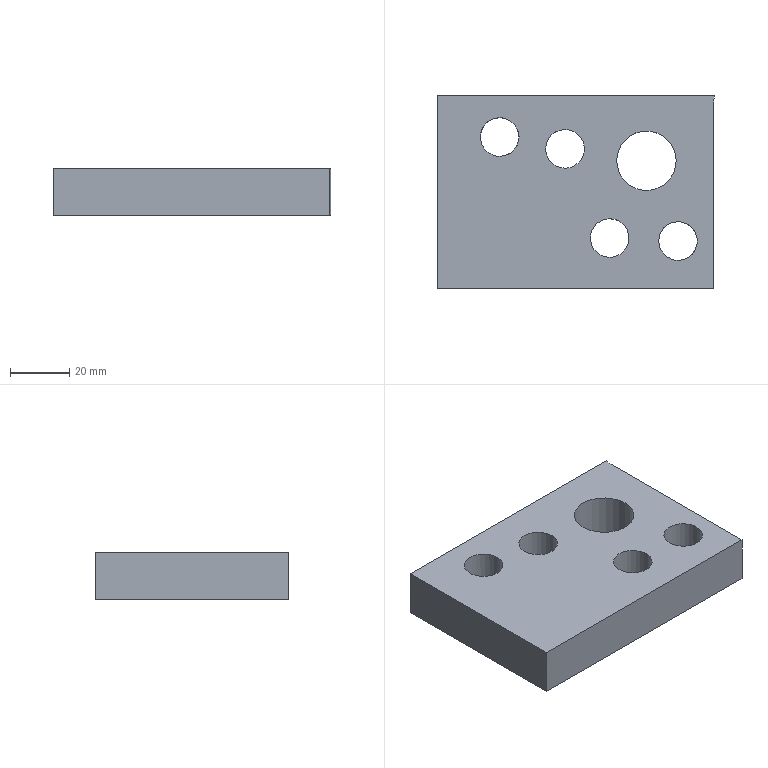Part | STEP file | gslz 2016.10.28-13_id746_x_t | 1 solid | 12 faces | box 93.344 x 65 x 16 mm | volume 83204 mm3 | plane 6 | cylinder 6 | commonest cylinder face diameters 13 x4 20 x1 22 x1
STEP:
#1=CARTESIAN_POINT('',(0.,0.,0.));
#2=DIRECTION('',(0.,0.,1.));
#3=DIRECTION('',(1.,0.,0.));
#4=AXIS2_PLACEMENT_3D('',#1,#2,#3);
#5=CARTESIAN_POINT('',(-1401.656,89.,-32.));
#6=VERTEX_POINT('',#5);
#7=CARTESIAN_POINT('',(-1495.,89.,-32.));
#8=VERTEX_POINT('',#7);
#9=CARTESIAN_POINT('',(-1374.,89.,-32.));
#10=DIRECTION('',(-1.,0.,0.));
#11=VECTOR('',#10,1.);
#12=LINE('',#9,#11);
#13=CARTESIAN_POINT('',(-1374.,128.728,-32.));
#14=DIRECTION('',(0.,0.,1.));
#15=DIRECTION('',(1.,0.,0.));
#16=AXIS2_PLACEMENT_3D('',#13,#14,#15);
#17=PLANE('',#16);
#18=CARTESIAN_POINT('',(0.,-39.728));
#19=DIRECTION('',(-1.,0.));
#20=VECTOR('',#19,1.);
#21=LINE('',#18,#20);
#22=(GEOMETRIC_REPRESENTATION_CONTEXT(2)PARAMETRIC_REPRESENTATION_CONTEXT()REPRESENTATION_CONTEXT('',''));
#23=DEFINITIONAL_REPRESENTATION('',(#21),#22);
#24=PCURVE('',#17,#23);
#25=CARTESIAN_POINT('',(-1448.,89.,-12.));
#26=DIRECTION('',(0.,-1.,0.));
#27=DIRECTION('',(0.,0.,-1.));
#28=AXIS2_PLACEMENT_3D('',#25,#26,#27);
#29=PLANE('',#28);
#30=CARTESIAN_POINT('',(20.,74.));
#31=DIRECTION('',(0.,-1.));
#32=VECTOR('',#31,1.);
#33=LINE('',#30,#32);
#34=(GEOMETRIC_REPRESENTATION_CONTEXT(2)PARAMETRIC_REPRESENTATION_CONTEXT()REPRESENTATION_CONTEXT('',''));
#35=DEFINITIONAL_REPRESENTATION('',(#33),#34);
#36=PCURVE('',#29,#35);
#37=SURFACE_CURVE('',#12,(#24,#36),.PCURVE_S1.);
#38=EDGE_CURVE('',#6,#8,#37,.T.);
#39=ORIENTED_EDGE('',*,*,#38,.T.);
#40=CARTESIAN_POINT('',(-1495.,24.,-32.));
#41=VERTEX_POINT('',#40);
#42=CARTESIAN_POINT('',(-1495.,220.,-32.));
#43=DIRECTION('',(0.,-1.,0.));
#44=VECTOR('',#43,1.);
#45=LINE('',#42,#44);
#46=CARTESIAN_POINT('',(-121.,91.272));
#47=DIRECTION('',(0.,-1.));
#48=VECTOR('',#47,1.);
#49=LINE('',#46,#48);
#50=(GEOMETRIC_REPRESENTATION_CONTEXT(2)PARAMETRIC_REPRESENTATION_CONTEXT()REPRESENTATION_CONTEXT('',''));
#51=DEFINITIONAL_REPRESENTATION('',(#49),#50);
#52=PCURVE('',#17,#51);
#53=CARTESIAN_POINT('',(-1495.,220.,-40.));
#54=DIRECTION('',(-1.,0.,0.));
#55=DIRECTION('',(0.,0.,1.));
#56=AXIS2_PLACEMENT_3D('',#53,#54,#55);
#57=PLANE('',#56);
#58=CARTESIAN_POINT('',(8.,0.));
#59=DIRECTION('',(0.,-1.));
#60=VECTOR('',#59,1.);
#61=LINE('',#58,#60);
#62=(GEOMETRIC_REPRESENTATION_CONTEXT(2)PARAMETRIC_REPRESENTATION_CONTEXT()REPRESENTATION_CONTEXT('',''));
#63=DEFINITIONAL_REPRESENTATION('',(#61),#62);
#64=PCURVE('',#57,#63);
#65=SURFACE_CURVE('',#45,(#52,#64),.PCURVE_S1.);
#66=EDGE_CURVE('',#8,#41,#65,.T.);
#67=ORIENTED_EDGE('',*,*,#66,.T.);
#68=CARTESIAN_POINT('',(-1402.,24.,-32.));
#69=VERTEX_POINT('',#68);
#70=CARTESIAN_POINT('',(-1490.,24.,-32.));
#71=DIRECTION('',(1.,0.,0.));
#72=VECTOR('',#71,1.);
#73=LINE('',#70,#72);
#74=CARTESIAN_POINT('',(-116.,-104.728));
#75=DIRECTION('',(1.,0.));
#76=VECTOR('',#75,1.);
#77=LINE('',#74,#76);
#78=(GEOMETRIC_REPRESENTATION_CONTEXT(2)PARAMETRIC_REPRESENTATION_CONTEXT()REPRESENTATION_CONTEXT('',''));
#79=DEFINITIONAL_REPRESENTATION('',(#77),#78);
#80=PCURVE('',#17,#79);
#81=CARTESIAN_POINT('',(-1490.,24.,-40.));
#82=DIRECTION('',(0.,-1.,0.));
#83=DIRECTION('',(1.,0.,0.));
#84=AXIS2_PLACEMENT_3D('',#81,#82,#83);
#85=PLANE('',#84);
#86=CARTESIAN_POINT('',(0.,8.));
#87=DIRECTION('',(1.,0.));
#88=VECTOR('',#87,1.);
#89=LINE('',#86,#88);
#90=(GEOMETRIC_REPRESENTATION_CONTEXT(2)PARAMETRIC_REPRESENTATION_CONTEXT()REPRESENTATION_CONTEXT('',''));
#91=DEFINITIONAL_REPRESENTATION('',(#89),#90);
#92=PCURVE('',#85,#91);
#93=SURFACE_CURVE('',#73,(#80,#92),.PCURVE_S1.);
#94=EDGE_CURVE('',#41,#69,#93,.T.);
#95=ORIENTED_EDGE('',*,*,#94,.T.);
#96=CARTESIAN_POINT('',(-1402.,86.272,-32.));
#97=VERTEX_POINT('',#96);
#98=CARTESIAN_POINT('',(-1402.,128.728,-32.));
#99=DIRECTION('',(0.,1.,0.));
#100=VECTOR('',#99,1.);
#101=LINE('',#98,#100);
#102=CARTESIAN_POINT('',(-28.,0.));
#103=DIRECTION('',(0.,1.));
#104=VECTOR('',#103,1.);
#105=LINE('',#102,#104);
#106=(GEOMETRIC_REPRESENTATION_CONTEXT(2)PARAMETRIC_REPRESENTATION_CONTEXT()REPRESENTATION_CONTEXT('',''));
#107=DEFINITIONAL_REPRESENTATION('',(#105),#106);
#108=PCURVE('',#17,#107);
#109=CARTESIAN_POINT('',(-1402.,30.,-40.));
#110=DIRECTION('',(1.,0.,0.));
#111=DIRECTION('',(0.,1.,0.));
#112=AXIS2_PLACEMENT_3D('',#109,#110,#111);
#113=PLANE('',#112);
#114=CARTESIAN_POINT('',(98.728,8.));
#115=DIRECTION('',(1.,0.));
#116=VECTOR('',#115,1.);
#117=LINE('',#114,#116);
#118=(GEOMETRIC_REPRESENTATION_CONTEXT(2)PARAMETRIC_REPRESENTATION_CONTEXT()REPRESENTATION_CONTEXT('',''));
#119=DEFINITIONAL_REPRESENTATION('',(#117),#118);
#120=PCURVE('',#113,#119);
#121=SURFACE_CURVE('',#101,(#108,#120),.PCURVE_S1.);
#122=EDGE_CURVE('',#69,#97,#121,.T.);
#123=ORIENTED_EDGE('',*,*,#122,.T.);
#124=CARTESIAN_POINT('',(-1391.,86.272,-32.));
#125=DIRECTION('',(0.,0.,-1.));
#126=DIRECTION('',(1.,0.,0.));
#127=AXIS2_PLACEMENT_3D('',#124,#125,#126);
#128=CIRCLE('',#127,11.);
#129=CARTESIAN_POINT('',(-6.,-42.456));
#130=CARTESIAN_POINT('',(-6.,-61.508));
#131=CARTESIAN_POINT('',(-22.5,-51.982));
#132=CARTESIAN_POINT('',(-39.,-42.456));
#133=CARTESIAN_POINT('',(-22.5,-32.93));
#134=CARTESIAN_POINT('',(-6.,-23.403));
#135=CARTESIAN_POINT('',(-6.,-42.456));
#136=(BOUNDED_CURVE()B_SPLINE_CURVE(2,(#129,#130,#131,#132,#133,#134,#135),.UNSPECIFIED.,.T.,.F.)B_SPLINE_CURVE_WITH_KNOTS((1,2,2,2,2,1),(-2.094,0.,2.094,4.189,6.283,8.378),.UNSPECIFIED.)CURVE()GEOMETRIC_REPRESENTATION_ITEM()RATIONAL_B_SPLINE_CURVE((1.,0.5,1.,0.5,1.,0.5,1.))REPRESENTATION_ITEM(''));
#137=(GEOMETRIC_REPRESENTATION_CONTEXT(2)PARAMETRIC_REPRESENTATION_CONTEXT()REPRESENTATION_CONTEXT('',''));
#138=DEFINITIONAL_REPRESENTATION('',(#136),#137);
#139=PCURVE('',#17,#138);
#140=CARTESIAN_POINT('',(-1391.,86.272,-40.));
#141=DIRECTION('',(0.,0.,1.));
#142=DIRECTION('',(1.,0.,0.));
#143=AXIS2_PLACEMENT_3D('',#140,#141,#142);
#144=CYLINDRICAL_SURFACE('',#143,11.);
#145=CARTESIAN_POINT('',(6.283,8.));
#146=DIRECTION('',(-1.,0.));
#147=VECTOR('',#146,1.);
#148=LINE('',#145,#147);
#149=(GEOMETRIC_REPRESENTATION_CONTEXT(2)PARAMETRIC_REPRESENTATION_CONTEXT()REPRESENTATION_CONTEXT('',''));
#150=DEFINITIONAL_REPRESENTATION('',(#148),#149);
#151=PCURVE('',#144,#150);
#152=SURFACE_CURVE('',#128,(#139,#151),.PCURVE_S1.);
#153=EDGE_CURVE('',#97,#6,#152,.T.);
#154=ORIENTED_EDGE('',*,*,#153,.T.);
#155=EDGE_LOOP('',(#39,#67,#95,#123,#154));
#156=FACE_BOUND('',#155,.T.);
#157=CARTESIAN_POINT('',(-1435.568,47.34,-32.));
#158=VERTEX_POINT('',#157);
#159=CARTESIAN_POINT('',(-1437.,41.,-32.));
#160=DIRECTION('',(0.,0.,-1.));
#161=DIRECTION('',(0.2202,0.9754,0.));
#162=AXIS2_PLACEMENT_3D('',#159,#160,#161);
#163=CIRCLE('',#162,6.5);
#164=CARTESIAN_POINT('',(-61.568,-81.388));
#165=CARTESIAN_POINT('',(-50.587,-83.867));
#166=CARTESIAN_POINT('',(-58.225,-92.138));
#167=CARTESIAN_POINT('',(-65.863,-100.409));
#168=CARTESIAN_POINT('',(-69.207,-89.658));
#169=CARTESIAN_POINT('',(-72.55,-78.908));
#170=CARTESIAN_POINT('',(-61.568,-81.388));
#171=(BOUNDED_CURVE()B_SPLINE_CURVE(2,(#164,#165,#166,#167,#168,#169,#170),.UNSPECIFIED.,.T.,.F.)B_SPLINE_CURVE_WITH_KNOTS((1,2,2,2,2,1),(-2.094,0.,2.094,4.189,6.283,8.378),.UNSPECIFIED.)CURVE()GEOMETRIC_REPRESENTATION_ITEM()RATIONAL_B_SPLINE_CURVE((1.,0.5,1.,0.5,1.,0.5,1.))REPRESENTATION_ITEM(''));
#172=(GEOMETRIC_REPRESENTATION_CONTEXT(2)PARAMETRIC_REPRESENTATION_CONTEXT()REPRESENTATION_CONTEXT('',''));
#173=DEFINITIONAL_REPRESENTATION('',(#171),#172);
#174=PCURVE('',#17,#173);
#175=CARTESIAN_POINT('',(-1437.,41.,-95.));
#176=DIRECTION('',(0.,0.,1.));
#177=DIRECTION('',(-0.2202,-0.9754,0.));
#178=AXIS2_PLACEMENT_3D('',#175,#176,#177);
#179=CYLINDRICAL_SURFACE('',#178,6.5);
#180=CARTESIAN_POINT('',(9.425,63.));
#181=DIRECTION('',(-1.,0.));
#182=VECTOR('',#181,1.);
#183=LINE('',#180,#182);
#184=(GEOMETRIC_REPRESENTATION_CONTEXT(2)PARAMETRIC_REPRESENTATION_CONTEXT()REPRESENTATION_CONTEXT('',''));
#185=DEFINITIONAL_REPRESENTATION('',(#183),#184);
#186=PCURVE('',#179,#185);
#187=SURFACE_CURVE('',#163,(#174,#186),.PCURVE_S1.);
#188=EDGE_CURVE('',#158,#158,#187,.T.);
#189=ORIENTED_EDGE('',*,*,#188,.T.);
#190=EDGE_LOOP('',(#189));
#191=FACE_BOUND('',#190,.T.);
#192=CARTESIAN_POINT('',(-1414.627,66.996,-32.));
#193=VERTEX_POINT('',#192);
#194=CARTESIAN_POINT('',(-1424.627,66.996,-32.));
#195=DIRECTION('',(0.,0.,1.));
#196=DIRECTION('',(1.,0.,0.));
#197=AXIS2_PLACEMENT_3D('',#194,#195,#196);
#198=CIRCLE('',#197,10.);
#199=CARTESIAN_POINT('',(-50.627,-61.732));
#200=DIRECTION('',(1.,0.));
#201=AXIS2_PLACEMENT_2D('',#199,#200);
#202=CIRCLE('',#201,10.);
#203=(GEOMETRIC_REPRESENTATION_CONTEXT(2)PARAMETRIC_REPRESENTATION_CONTEXT()REPRESENTATION_CONTEXT('',''));
#204=DEFINITIONAL_REPRESENTATION('',(#202),#203);
#205=PCURVE('',#17,#204);
#206=CARTESIAN_POINT('',(-1424.627,66.996,-82.));
#207=DIRECTION('',(0.,0.,1.));
#208=DIRECTION('',(1.,0.,0.));
#209=AXIS2_PLACEMENT_3D('',#206,#207,#208);
#210=CYLINDRICAL_SURFACE('',#209,10.);
#211=CARTESIAN_POINT('',(0.,50.));
#212=DIRECTION('',(1.,0.));
#213=VECTOR('',#212,1.);
#214=LINE('',#211,#213);
#215=(GEOMETRIC_REPRESENTATION_CONTEXT(2)PARAMETRIC_REPRESENTATION_CONTEXT()REPRESENTATION_CONTEXT('',''));
#216=DEFINITIONAL_REPRESENTATION('',(#214),#215);
#217=PCURVE('',#210,#216);
#218=SURFACE_CURVE('',#198,(#205,#217),.PCURVE_S1.);
#219=EDGE_CURVE('',#193,#193,#218,.T.);
#220=ORIENTED_EDGE('',*,*,#219,.F.);
#221=EDGE_LOOP('',(#220));
#222=FACE_BOUND('',#221,.T.);
#223=CARTESIAN_POINT('',(-1467.5,75.,-32.));
#224=VERTEX_POINT('',#223);
#225=CARTESIAN_POINT('',(-1475.091,68.592,-32.));
#226=VERTEX_POINT('',#225);
#227=CARTESIAN_POINT('',(-1474.,75.,-32.));
#228=DIRECTION('',(0.,0.,1.));
#229=DIRECTION('',(1.,0.,0.));
#230=AXIS2_PLACEMENT_3D('',#227,#228,#229);
#231=CIRCLE('',#230,6.5);
#232=CARTESIAN_POINT('',(-100.,-53.728));
#233=DIRECTION('',(1.,0.));
#234=AXIS2_PLACEMENT_2D('',#232,#233);
#235=CIRCLE('',#234,6.5);
#236=(GEOMETRIC_REPRESENTATION_CONTEXT(2)PARAMETRIC_REPRESENTATION_CONTEXT()REPRESENTATION_CONTEXT('',''));
#237=DEFINITIONAL_REPRESENTATION('',(#235),#236);
#238=PCURVE('',#17,#237);
#239=CARTESIAN_POINT('',(-1474.,75.,-0.5408));
#240=DIRECTION('',(0.,0.,-1.));
#241=DIRECTION('',(-1.,0.,0.));
#242=AXIS2_PLACEMENT_3D('',#239,#240,#241);
#243=CYLINDRICAL_SURFACE('',#242,6.5);
#244=CARTESIAN_POINT('',(9.425,31.459));
#245=DIRECTION('',(-1.,0.));
#246=VECTOR('',#245,1.);
#247=LINE('',#244,#246);
#248=(GEOMETRIC_REPRESENTATION_CONTEXT(2)PARAMETRIC_REPRESENTATION_CONTEXT()REPRESENTATION_CONTEXT('',''));
#249=DEFINITIONAL_REPRESENTATION('',(#247),#248);
#250=PCURVE('',#243,#249);
#251=SURFACE_CURVE('',#231,(#238,#250),.PCURVE_S1.);
#252=EDGE_CURVE('',#224,#226,#251,.T.);
#253=ORIENTED_EDGE('',*,*,#252,.F.);
#254=CARTESIAN_POINT('',(-1474.,75.,-32.));
#255=DIRECTION('',(0.,0.,1.));
#256=DIRECTION('',(1.,0.,0.));
#257=AXIS2_PLACEMENT_3D('',#254,#255,#256);
#258=CIRCLE('',#257,6.5);
#259=CARTESIAN_POINT('',(-100.,-53.728));
#260=DIRECTION('',(1.,0.));
#261=AXIS2_PLACEMENT_2D('',#259,#260);
#262=CIRCLE('',#261,6.5);
#263=(GEOMETRIC_REPRESENTATION_CONTEXT(2)PARAMETRIC_REPRESENTATION_CONTEXT()REPRESENTATION_CONTEXT('',''));
#264=DEFINITIONAL_REPRESENTATION('',(#262),#263);
#265=PCURVE('',#17,#264);
#266=CARTESIAN_POINT('',(15.708,31.459));
#267=DIRECTION('',(-1.,0.));
#268=VECTOR('',#267,1.);
#269=LINE('',#266,#268);
#270=(GEOMETRIC_REPRESENTATION_CONTEXT(2)PARAMETRIC_REPRESENTATION_CONTEXT()REPRESENTATION_CONTEXT('',''));
#271=DEFINITIONAL_REPRESENTATION('',(#269),#270);
#272=PCURVE('',#243,#271);
#273=SURFACE_CURVE('',#258,(#265,#272),.PCURVE_S1.);
#274=EDGE_CURVE('',#226,#224,#273,.T.);
#275=ORIENTED_EDGE('',*,*,#274,.F.);
#276=EDGE_LOOP('',(#253,#275));
#277=FACE_BOUND('',#276,.T.);
#278=CARTESIAN_POINT('',(-1450.568,77.34,-32.));
#279=VERTEX_POINT('',#278);
#280=CARTESIAN_POINT('',(-1452.,71.,-32.));
#281=DIRECTION('',(0.,0.,-1.));
#282=DIRECTION('',(0.2202,0.9754,0.));
#283=AXIS2_PLACEMENT_3D('',#280,#281,#282);
#284=CIRCLE('',#283,6.5);
#285=CARTESIAN_POINT('',(-76.568,-51.388));
#286=CARTESIAN_POINT('',(-65.587,-53.867));
#287=CARTESIAN_POINT('',(-73.225,-62.138));
#288=CARTESIAN_POINT('',(-80.863,-70.409));
#289=CARTESIAN_POINT('',(-84.207,-59.658));
#290=CARTESIAN_POINT('',(-87.55,-48.908));
#291=CARTESIAN_POINT('',(-76.568,-51.388));
#292=(BOUNDED_CURVE()B_SPLINE_CURVE(2,(#285,#286,#287,#288,#289,#290,#291),.UNSPECIFIED.,.T.,.F.)B_SPLINE_CURVE_WITH_KNOTS((1,2,2,2,2,1),(-2.094,0.,2.094,4.189,6.283,8.378),.UNSPECIFIED.)CURVE()GEOMETRIC_REPRESENTATION_ITEM()RATIONAL_B_SPLINE_CURVE((1.,0.5,1.,0.5,1.,0.5,1.))REPRESENTATION_ITEM(''));
#293=(GEOMETRIC_REPRESENTATION_CONTEXT(2)PARAMETRIC_REPRESENTATION_CONTEXT()REPRESENTATION_CONTEXT('',''));
#294=DEFINITIONAL_REPRESENTATION('',(#292),#293);
#295=PCURVE('',#17,#294);
#296=CARTESIAN_POINT('',(-1452.,71.,-95.));
#297=DIRECTION('',(0.,0.,1.));
#298=DIRECTION('',(-0.2202,-0.9754,0.));
#299=AXIS2_PLACEMENT_3D('',#296,#297,#298);
#300=CYLINDRICAL_SURFACE('',#299,6.5);
#301=CARTESIAN_POINT('',(9.425,63.));
#302=DIRECTION('',(-1.,0.));
#303=VECTOR('',#302,1.);
#304=LINE('',#301,#303);
#305=(GEOMETRIC_REPRESENTATION_CONTEXT(2)PARAMETRIC_REPRESENTATION_CONTEXT()REPRESENTATION_CONTEXT('',''));
#306=DEFINITIONAL_REPRESENTATION('',(#304),#305);
#307=PCURVE('',#300,#306);
#308=SURFACE_CURVE('',#284,(#295,#307),.PCURVE_S1.);
#309=EDGE_CURVE('',#279,#279,#308,.T.);
#310=ORIENTED_EDGE('',*,*,#309,.T.);
#311=EDGE_LOOP('',(#310));
#312=FACE_BOUND('',#311,.T.);
#313=CARTESIAN_POINT('',(-1407.5,40.,-32.));
#314=VERTEX_POINT('',#313);
#315=CARTESIAN_POINT('',(-1415.091,33.592,-32.));
#316=VERTEX_POINT('',#315);
#317=CARTESIAN_POINT('',(-1414.,40.,-32.));
#318=DIRECTION('',(0.,0.,1.));
#319=DIRECTION('',(1.,0.,0.));
#320=AXIS2_PLACEMENT_3D('',#317,#318,#319);
#321=CIRCLE('',#320,6.5);
#322=CARTESIAN_POINT('',(-40.,-88.728));
#323=DIRECTION('',(1.,0.));
#324=AXIS2_PLACEMENT_2D('',#322,#323);
#325=CIRCLE('',#324,6.5);
#326=(GEOMETRIC_REPRESENTATION_CONTEXT(2)PARAMETRIC_REPRESENTATION_CONTEXT()REPRESENTATION_CONTEXT('',''));
#327=DEFINITIONAL_REPRESENTATION('',(#325),#326);
#328=PCURVE('',#17,#327);
#329=CARTESIAN_POINT('',(-1414.,40.,-0.5408));
#330=DIRECTION('',(0.,0.,-1.));
#331=DIRECTION('',(-1.,0.,0.));
#332=AXIS2_PLACEMENT_3D('',#329,#330,#331);
#333=CYLINDRICAL_SURFACE('',#332,6.5);
#334=CARTESIAN_POINT('',(9.425,31.459));
#335=DIRECTION('',(-1.,0.));
#336=VECTOR('',#335,1.);
#337=LINE('',#334,#336);
#338=(GEOMETRIC_REPRESENTATION_CONTEXT(2)PARAMETRIC_REPRESENTATION_CONTEXT()REPRESENTATION_CONTEXT('',''));
#339=DEFINITIONAL_REPRESENTATION('',(#337),#338);
#340=PCURVE('',#333,#339);
#341=SURFACE_CURVE('',#321,(#328,#340),.PCURVE_S1.);
#342=EDGE_CURVE('',#314,#316,#341,.T.);
#343=ORIENTED_EDGE('',*,*,#342,.F.);
#344=CARTESIAN_POINT('',(-1414.,40.,-32.));
#345=DIRECTION('',(0.,0.,1.));
#346=DIRECTION('',(1.,0.,0.));
#347=AXIS2_PLACEMENT_3D('',#344,#345,#346);
#348=CIRCLE('',#347,6.5);
#349=CARTESIAN_POINT('',(-40.,-88.728));
#350=DIRECTION('',(1.,0.));
#351=AXIS2_PLACEMENT_2D('',#349,#350);
#352=CIRCLE('',#351,6.5);
#353=(GEOMETRIC_REPRESENTATION_CONTEXT(2)PARAMETRIC_REPRESENTATION_CONTEXT()REPRESENTATION_CONTEXT('',''));
#354=DEFINITIONAL_REPRESENTATION('',(#352),#353);
#355=PCURVE('',#17,#354);
#356=CARTESIAN_POINT('',(15.708,31.459));
#357=DIRECTION('',(-1.,0.));
#358=VECTOR('',#357,1.);
#359=LINE('',#356,#358);
#360=(GEOMETRIC_REPRESENTATION_CONTEXT(2)PARAMETRIC_REPRESENTATION_CONTEXT()REPRESENTATION_CONTEXT('',''));
#361=DEFINITIONAL_REPRESENTATION('',(#359),#360);
#362=PCURVE('',#333,#361);
#363=SURFACE_CURVE('',#348,(#355,#362),.PCURVE_S1.);
#364=EDGE_CURVE('',#316,#314,#363,.T.);
#365=ORIENTED_EDGE('',*,*,#364,.F.);
#366=EDGE_LOOP('',(#343,#365));
#367=FACE_BOUND('',#366,.T.);
#368=ADVANCED_FACE('',(#156,#191,#222,#277,#312,#367),#17,.T.);
#369=CARTESIAN_POINT('',(-1415.091,33.592,-48.));
#370=VERTEX_POINT('',#369);
#371=CARTESIAN_POINT('',(-1414.,40.,-48.));
#372=DIRECTION('',(0.,0.,1.));
#373=DIRECTION('',(-0.1678,-0.9858,0.));
#374=AXIS2_PLACEMENT_3D('',#371,#372,#373);
#375=CIRCLE('',#374,6.5);
#376=CARTESIAN_POINT('',(-1374.,128.728,-48.));
#377=DIRECTION('',(0.,0.,1.));
#378=DIRECTION('',(1.,0.,0.));
#379=AXIS2_PLACEMENT_3D('',#376,#377,#378);
#380=PLANE('',#379);
#381=CARTESIAN_POINT('',(-40.,-88.728));
#382=DIRECTION('',(-0.1678,-0.9858));
#383=AXIS2_PLACEMENT_2D('',#381,#382);
#384=CIRCLE('',#383,6.5);
#385=(GEOMETRIC_REPRESENTATION_CONTEXT(2)PARAMETRIC_REPRESENTATION_CONTEXT()REPRESENTATION_CONTEXT('',''));
#386=DEFINITIONAL_REPRESENTATION('',(#384),#385);
#387=PCURVE('',#380,#386);
#388=CARTESIAN_POINT('',(11.164,47.459));
#389=DIRECTION('',(-1.,0.));
#390=VECTOR('',#389,1.);
#391=LINE('',#388,#390);
#392=(GEOMETRIC_REPRESENTATION_CONTEXT(2)PARAMETRIC_REPRESENTATION_CONTEXT()REPRESENTATION_CONTEXT('',''));
#393=DEFINITIONAL_REPRESENTATION('',(#391),#392);
#394=PCURVE('',#333,#393);
#395=SURFACE_CURVE('',#375,(#387,#394),.PCURVE_S1.);
#396=EDGE_CURVE('',#370,#370,#395,.T.);
#397=ORIENTED_EDGE('',*,*,#396,.T.);
#398=EDGE_LOOP('',(#397));
#399=FACE_BOUND('',#398,.T.);
#400=CARTESIAN_POINT('',(-1435.568,47.34,-48.));
#401=VERTEX_POINT('',#400);
#402=CARTESIAN_POINT('',(-1437.,41.,-48.));
#403=DIRECTION('',(0.,0.,1.));
#404=DIRECTION('',(0.2202,0.9754,0.));
#405=AXIS2_PLACEMENT_3D('',#402,#403,#404);
#406=CIRCLE('',#405,6.5);
#407=CARTESIAN_POINT('',(-63.,-87.728));
#408=DIRECTION('',(0.2202,0.9754));
#409=AXIS2_PLACEMENT_2D('',#407,#408);
#410=CIRCLE('',#409,6.5);
#411=(GEOMETRIC_REPRESENTATION_CONTEXT(2)PARAMETRIC_REPRESENTATION_CONTEXT()REPRESENTATION_CONTEXT('',''));
#412=DEFINITIONAL_REPRESENTATION('',(#410),#411);
#413=PCURVE('',#380,#412);
#414=CARTESIAN_POINT('',(3.142,47.));
#415=DIRECTION('',(1.,0.));
#416=VECTOR('',#415,1.);
#417=LINE('',#414,#416);
#418=(GEOMETRIC_REPRESENTATION_CONTEXT(2)PARAMETRIC_REPRESENTATION_CONTEXT()REPRESENTATION_CONTEXT('',''));
#419=DEFINITIONAL_REPRESENTATION('',(#417),#418);
#420=PCURVE('',#179,#419);
#421=SURFACE_CURVE('',#406,(#413,#420),.PCURVE_S1.);
#422=EDGE_CURVE('',#401,#401,#421,.T.);
#423=ORIENTED_EDGE('',*,*,#422,.T.);
#424=EDGE_LOOP('',(#423));
#425=FACE_BOUND('',#424,.T.);
#426=CARTESIAN_POINT('',(-1450.568,77.34,-48.));
#427=VERTEX_POINT('',#426);
#428=CARTESIAN_POINT('',(-1452.,71.,-48.));
#429=DIRECTION('',(0.,0.,1.));
#430=DIRECTION('',(0.2202,0.9754,0.));
#431=AXIS2_PLACEMENT_3D('',#428,#429,#430);
#432=CIRCLE('',#431,6.5);
#433=CARTESIAN_POINT('',(-78.,-57.728));
#434=DIRECTION('',(0.2202,0.9754));
#435=AXIS2_PLACEMENT_2D('',#433,#434);
#436=CIRCLE('',#435,6.5);
#437=(GEOMETRIC_REPRESENTATION_CONTEXT(2)PARAMETRIC_REPRESENTATION_CONTEXT()REPRESENTATION_CONTEXT('',''));
#438=DEFINITIONAL_REPRESENTATION('',(#436),#437);
#439=PCURVE('',#380,#438);
#440=CARTESIAN_POINT('',(3.142,47.));
#441=DIRECTION('',(1.,0.));
#442=VECTOR('',#441,1.);
#443=LINE('',#440,#442);
#444=(GEOMETRIC_REPRESENTATION_CONTEXT(2)PARAMETRIC_REPRESENTATION_CONTEXT()REPRESENTATION_CONTEXT('',''));
#445=DEFINITIONAL_REPRESENTATION('',(#443),#444);
#446=PCURVE('',#300,#445);
#447=SURFACE_CURVE('',#432,(#439,#446),.PCURVE_S1.);
#448=EDGE_CURVE('',#427,#427,#447,.T.);
#449=ORIENTED_EDGE('',*,*,#448,.T.);
#450=EDGE_LOOP('',(#449));
#451=FACE_BOUND('',#450,.T.);
#452=CARTESIAN_POINT('',(-1475.091,68.592,-48.));
#453=VERTEX_POINT('',#452);
#454=CARTESIAN_POINT('',(-1474.,75.,-48.));
#455=DIRECTION('',(0.,0.,1.));
#456=DIRECTION('',(-0.1678,-0.9858,0.));
#457=AXIS2_PLACEMENT_3D('',#454,#455,#456);
#458=CIRCLE('',#457,6.5);
#459=CARTESIAN_POINT('',(-100.,-53.728));
#460=DIRECTION('',(-0.1678,-0.9858));
#461=AXIS2_PLACEMENT_2D('',#459,#460);
#462=CIRCLE('',#461,6.5);
#463=(GEOMETRIC_REPRESENTATION_CONTEXT(2)PARAMETRIC_REPRESENTATION_CONTEXT()REPRESENTATION_CONTEXT('',''));
#464=DEFINITIONAL_REPRESENTATION('',(#462),#463);
#465=PCURVE('',#380,#464);
#466=CARTESIAN_POINT('',(11.164,47.459));
#467=DIRECTION('',(-1.,0.));
#468=VECTOR('',#467,1.);
#469=LINE('',#466,#468);
#470=(GEOMETRIC_REPRESENTATION_CONTEXT(2)PARAMETRIC_REPRESENTATION_CONTEXT()REPRESENTATION_CONTEXT('',''));
#471=DEFINITIONAL_REPRESENTATION('',(#469),#470);
#472=PCURVE('',#243,#471);
#473=SURFACE_CURVE('',#458,(#465,#472),.PCURVE_S1.);
#474=EDGE_CURVE('',#453,#453,#473,.T.);
#475=ORIENTED_EDGE('',*,*,#474,.T.);
#476=EDGE_LOOP('',(#475));
#477=FACE_BOUND('',#476,.T.);
#478=CARTESIAN_POINT('',(-1414.627,66.996,-48.));
#479=VERTEX_POINT('',#478);
#480=CARTESIAN_POINT('',(-1424.627,66.996,-48.));
#481=DIRECTION('',(0.,0.,1.));
#482=DIRECTION('',(1.,0.,0.));
#483=AXIS2_PLACEMENT_3D('',#480,#481,#482);
#484=CIRCLE('',#483,10.);
#485=CARTESIAN_POINT('',(-50.627,-61.732));
#486=DIRECTION('',(1.,0.));
#487=AXIS2_PLACEMENT_2D('',#485,#486);
#488=CIRCLE('',#487,10.);
#489=(GEOMETRIC_REPRESENTATION_CONTEXT(2)PARAMETRIC_REPRESENTATION_CONTEXT()REPRESENTATION_CONTEXT('',''));
#490=DEFINITIONAL_REPRESENTATION('',(#488),#489);
#491=PCURVE('',#380,#490);
#492=CARTESIAN_POINT('',(0.,34.));
#493=DIRECTION('',(1.,0.));
#494=VECTOR('',#493,1.);
#495=LINE('',#492,#494);
#496=(GEOMETRIC_REPRESENTATION_CONTEXT(2)PARAMETRIC_REPRESENTATION_CONTEXT()REPRESENTATION_CONTEXT('',''));
#497=DEFINITIONAL_REPRESENTATION('',(#495),#496);
#498=PCURVE('',#210,#497);
#499=SURFACE_CURVE('',#484,(#491,#498),.PCURVE_S1.);
#500=EDGE_CURVE('',#479,#479,#499,.T.);
#501=ORIENTED_EDGE('',*,*,#500,.T.);
#502=EDGE_LOOP('',(#501));
#503=FACE_BOUND('',#502,.T.);
#504=CARTESIAN_POINT('',(-1495.,89.,-48.));
#505=VERTEX_POINT('',#504);
#506=CARTESIAN_POINT('',(-1495.,24.,-48.));
#507=VERTEX_POINT('',#506);
#508=CARTESIAN_POINT('',(-1495.,220.,-48.));
#509=DIRECTION('',(0.,-1.,0.));
#510=VECTOR('',#509,1.);
#511=LINE('',#508,#510);
#512=CARTESIAN_POINT('',(-121.,91.272));
#513=DIRECTION('',(0.,-1.));
#514=VECTOR('',#513,1.);
#515=LINE('',#512,#514);
#516=(GEOMETRIC_REPRESENTATION_CONTEXT(2)PARAMETRIC_REPRESENTATION_CONTEXT()REPRESENTATION_CONTEXT('',''));
#517=DEFINITIONAL_REPRESENTATION('',(#515),#516);
#518=PCURVE('',#380,#517);
#519=CARTESIAN_POINT('',(-8.,0.));
#520=DIRECTION('',(0.,-1.));
#521=VECTOR('',#520,1.);
#522=LINE('',#519,#521);
#523=(GEOMETRIC_REPRESENTATION_CONTEXT(2)PARAMETRIC_REPRESENTATION_CONTEXT()REPRESENTATION_CONTEXT('',''));
#524=DEFINITIONAL_REPRESENTATION('',(#522),#523);
#525=PCURVE('',#57,#524);
#526=SURFACE_CURVE('',#511,(#518,#525),.PCURVE_S1.);
#527=EDGE_CURVE('',#505,#507,#526,.T.);
#528=ORIENTED_EDGE('',*,*,#527,.F.);
#529=CARTESIAN_POINT('',(-1401.656,89.,-48.));
#530=VERTEX_POINT('',#529);
#531=CARTESIAN_POINT('',(-1374.,89.,-48.));
#532=DIRECTION('',(-1.,0.,0.));
#533=VECTOR('',#532,1.);
#534=LINE('',#531,#533);
#535=CARTESIAN_POINT('',(0.,-39.728));
#536=DIRECTION('',(-1.,0.));
#537=VECTOR('',#536,1.);
#538=LINE('',#535,#537);
#539=(GEOMETRIC_REPRESENTATION_CONTEXT(2)PARAMETRIC_REPRESENTATION_CONTEXT()REPRESENTATION_CONTEXT('',''));
#540=DEFINITIONAL_REPRESENTATION('',(#538),#539);
#541=PCURVE('',#380,#540);
#542=CARTESIAN_POINT('',(36.,74.));
#543=DIRECTION('',(0.,-1.));
#544=VECTOR('',#543,1.);
#545=LINE('',#542,#544);
#546=(GEOMETRIC_REPRESENTATION_CONTEXT(2)PARAMETRIC_REPRESENTATION_CONTEXT()REPRESENTATION_CONTEXT('',''));
#547=DEFINITIONAL_REPRESENTATION('',(#545),#546);
#548=PCURVE('',#29,#547);
#549=SURFACE_CURVE('',#534,(#541,#548),.PCURVE_S1.);
#550=EDGE_CURVE('',#530,#505,#549,.T.);
#551=ORIENTED_EDGE('',*,*,#550,.F.);
#552=CARTESIAN_POINT('',(-1402.,86.272,-48.));
#553=VERTEX_POINT('',#552);
#554=CARTESIAN_POINT('',(-1391.,86.272,-48.));
#555=DIRECTION('',(0.,0.,-1.));
#556=DIRECTION('',(1.,0.,0.));
#557=AXIS2_PLACEMENT_3D('',#554,#555,#556);
#558=CIRCLE('',#557,11.);
#559=CARTESIAN_POINT('',(-6.,-42.456));
#560=CARTESIAN_POINT('',(-6.,-61.508));
#561=CARTESIAN_POINT('',(-22.5,-51.982));
#562=CARTESIAN_POINT('',(-39.,-42.456));
#563=CARTESIAN_POINT('',(-22.5,-32.93));
#564=CARTESIAN_POINT('',(-6.,-23.403));
#565=CARTESIAN_POINT('',(-6.,-42.456));
#566=(BOUNDED_CURVE()B_SPLINE_CURVE(2,(#559,#560,#561,#562,#563,#564,#565),.UNSPECIFIED.,.T.,.F.)B_SPLINE_CURVE_WITH_KNOTS((1,2,2,2,2,1),(-2.094,0.,2.094,4.189,6.283,8.378),.UNSPECIFIED.)CURVE()GEOMETRIC_REPRESENTATION_ITEM()RATIONAL_B_SPLINE_CURVE((1.,0.5,1.,0.5,1.,0.5,1.))REPRESENTATION_ITEM(''));
#567=(GEOMETRIC_REPRESENTATION_CONTEXT(2)PARAMETRIC_REPRESENTATION_CONTEXT()REPRESENTATION_CONTEXT('',''));
#568=DEFINITIONAL_REPRESENTATION('',(#566),#567);
#569=PCURVE('',#380,#568);
#570=CARTESIAN_POINT('',(6.283,-8.));
#571=DIRECTION('',(-1.,0.));
#572=VECTOR('',#571,1.);
#573=LINE('',#570,#572);
#574=(GEOMETRIC_REPRESENTATION_CONTEXT(2)PARAMETRIC_REPRESENTATION_CONTEXT()REPRESENTATION_CONTEXT('',''));
#575=DEFINITIONAL_REPRESENTATION('',(#573),#574);
#576=PCURVE('',#144,#575);
#577=SURFACE_CURVE('',#558,(#569,#576),.PCURVE_S1.);
#578=EDGE_CURVE('',#553,#530,#577,.T.);
#579=ORIENTED_EDGE('',*,*,#578,.F.);
#580=CARTESIAN_POINT('',(-1402.,24.,-48.));
#581=VERTEX_POINT('',#580);
#582=CARTESIAN_POINT('',(-1402.,128.728,-48.));
#583=DIRECTION('',(0.,1.,0.));
#584=VECTOR('',#583,1.);
#585=LINE('',#582,#584);
#586=CARTESIAN_POINT('',(-28.,0.));
#587=DIRECTION('',(0.,1.));
#588=VECTOR('',#587,1.);
#589=LINE('',#586,#588);
#590=(GEOMETRIC_REPRESENTATION_CONTEXT(2)PARAMETRIC_REPRESENTATION_CONTEXT()REPRESENTATION_CONTEXT('',''));
#591=DEFINITIONAL_REPRESENTATION('',(#589),#590);
#592=PCURVE('',#380,#591);
#593=CARTESIAN_POINT('',(98.728,-8.));
#594=DIRECTION('',(1.,0.));
#595=VECTOR('',#594,1.);
#596=LINE('',#593,#595);
#597=(GEOMETRIC_REPRESENTATION_CONTEXT(2)PARAMETRIC_REPRESENTATION_CONTEXT()REPRESENTATION_CONTEXT('',''));
#598=DEFINITIONAL_REPRESENTATION('',(#596),#597);
#599=PCURVE('',#113,#598);
#600=SURFACE_CURVE('',#585,(#592,#599),.PCURVE_S1.);
#601=EDGE_CURVE('',#581,#553,#600,.T.);
#602=ORIENTED_EDGE('',*,*,#601,.F.);
#603=CARTESIAN_POINT('',(-1490.,24.,-48.));
#604=DIRECTION('',(1.,0.,0.));
#605=VECTOR('',#604,1.);
#606=LINE('',#603,#605);
#607=CARTESIAN_POINT('',(-116.,-104.728));
#608=DIRECTION('',(1.,0.));
#609=VECTOR('',#608,1.);
#610=LINE('',#607,#609);
#611=(GEOMETRIC_REPRESENTATION_CONTEXT(2)PARAMETRIC_REPRESENTATION_CONTEXT()REPRESENTATION_CONTEXT('',''));
#612=DEFINITIONAL_REPRESENTATION('',(#610),#611);
#613=PCURVE('',#380,#612);
#614=CARTESIAN_POINT('',(0.,-8.));
#615=DIRECTION('',(1.,0.));
#616=VECTOR('',#615,1.);
#617=LINE('',#614,#616);
#618=(GEOMETRIC_REPRESENTATION_CONTEXT(2)PARAMETRIC_REPRESENTATION_CONTEXT()REPRESENTATION_CONTEXT('',''));
#619=DEFINITIONAL_REPRESENTATION('',(#617),#618);
#620=PCURVE('',#85,#619);
#621=SURFACE_CURVE('',#606,(#613,#620),.PCURVE_S1.);
#622=EDGE_CURVE('',#507,#581,#621,.T.);
#623=ORIENTED_EDGE('',*,*,#622,.F.);
#624=EDGE_LOOP('',(#528,#551,#579,#602,#623));
#625=FACE_BOUND('',#624,.T.);
#626=ADVANCED_FACE('',(#399,#425,#451,#477,#503,#625),#380,.F.);
#627=ORIENTED_EDGE('',*,*,#578,.F.);
#628=CARTESIAN_POINT('',(-1402.,86.272,-40.));
#629=DIRECTION('',(0.,0.,1.));
#630=VECTOR('',#629,1.);
#631=LINE('',#628,#630);
#632=CARTESIAN_POINT('',(3.142,0.));
#633=DIRECTION('',(0.,1.));
#634=VECTOR('',#633,1.);
#635=LINE('',#632,#634);
#636=(GEOMETRIC_REPRESENTATION_CONTEXT(2)PARAMETRIC_REPRESENTATION_CONTEXT()REPRESENTATION_CONTEXT('',''));
#637=DEFINITIONAL_REPRESENTATION('',(#635),#636);
#638=PCURVE('',#144,#637);
#639=CARTESIAN_POINT('',(56.272,0.));
#640=DIRECTION('',(0.,1.));
#641=VECTOR('',#640,1.);
#642=LINE('',#639,#641);
#643=(GEOMETRIC_REPRESENTATION_CONTEXT(2)PARAMETRIC_REPRESENTATION_CONTEXT()REPRESENTATION_CONTEXT('',''));
#644=DEFINITIONAL_REPRESENTATION('',(#642),#643);
#645=PCURVE('',#113,#644);
#646=SURFACE_CURVE('',#631,(#638,#645),.PCURVE_S1.);
#647=EDGE_CURVE('',#553,#97,#646,.T.);
#648=ORIENTED_EDGE('',*,*,#647,.T.);
#649=ORIENTED_EDGE('',*,*,#153,.T.);
#650=CARTESIAN_POINT('',(-1401.656,89.,-40.));
#651=DIRECTION('',(0.,0.,1.));
#652=VECTOR('',#651,1.);
#653=LINE('',#650,#652);
#654=CARTESIAN_POINT('',(2.891,0.));
#655=DIRECTION('',(0.,1.));
#656=VECTOR('',#655,1.);
#657=LINE('',#654,#656);
#658=(GEOMETRIC_REPRESENTATION_CONTEXT(2)PARAMETRIC_REPRESENTATION_CONTEXT()REPRESENTATION_CONTEXT('',''));
#659=DEFINITIONAL_REPRESENTATION('',(#657),#658);
#660=PCURVE('',#144,#659);
#661=CARTESIAN_POINT('',(28.,46.344));
#662=DIRECTION('',(-1.,0.));
#663=VECTOR('',#662,1.);
#664=LINE('',#661,#663);
#665=(GEOMETRIC_REPRESENTATION_CONTEXT(2)PARAMETRIC_REPRESENTATION_CONTEXT()REPRESENTATION_CONTEXT('',''));
#666=DEFINITIONAL_REPRESENTATION('',(#664),#665);
#667=PCURVE('',#29,#666);
#668=SURFACE_CURVE('',#653,(#660,#667),.PCURVE_S1.);
#669=EDGE_CURVE('',#530,#6,#668,.T.);
#670=ORIENTED_EDGE('',*,*,#669,.F.);
#671=EDGE_LOOP('',(#627,#648,#649,#670));
#672=FACE_BOUND('',#671,.F.);
#673=ADVANCED_FACE('',(#672),#144,.F.);
#674=ORIENTED_EDGE('',*,*,#122,.F.);
#675=CARTESIAN_POINT('',(-1402.,24.,-40.));
#676=DIRECTION('',(0.,0.,1.));
#677=VECTOR('',#676,1.);
#678=LINE('',#675,#677);
#679=CARTESIAN_POINT('',(-6.,0.));
#680=DIRECTION('',(0.,1.));
#681=VECTOR('',#680,1.);
#682=LINE('',#679,#681);
#683=(GEOMETRIC_REPRESENTATION_CONTEXT(2)PARAMETRIC_REPRESENTATION_CONTEXT()REPRESENTATION_CONTEXT('',''));
#684=DEFINITIONAL_REPRESENTATION('',(#682),#683);
#685=PCURVE('',#113,#684);
#686=CARTESIAN_POINT('',(88.,0.));
#687=DIRECTION('',(0.,1.));
#688=VECTOR('',#687,1.);
#689=LINE('',#686,#688);
#690=(GEOMETRIC_REPRESENTATION_CONTEXT(2)PARAMETRIC_REPRESENTATION_CONTEXT()REPRESENTATION_CONTEXT('',''));
#691=DEFINITIONAL_REPRESENTATION('',(#689),#690);
#692=PCURVE('',#85,#691);
#693=SURFACE_CURVE('',#678,(#685,#692),.PCURVE_S1.);
#694=EDGE_CURVE('',#581,#69,#693,.T.);
#695=ORIENTED_EDGE('',*,*,#694,.F.);
#696=ORIENTED_EDGE('',*,*,#601,.T.);
#697=ORIENTED_EDGE('',*,*,#647,.T.);
#698=EDGE_LOOP('',(#674,#695,#696,#697));
#699=FACE_BOUND('',#698,.T.);
#700=ADVANCED_FACE('',(#699),#113,.T.);
#701=ORIENTED_EDGE('',*,*,#94,.F.);
#702=CARTESIAN_POINT('',(-1495.,24.,-40.));
#703=DIRECTION('',(0.,0.,1.));
#704=VECTOR('',#703,1.);
#705=LINE('',#702,#704);
#706=CARTESIAN_POINT('',(-5.,0.));
#707=DIRECTION('',(0.,1.));
#708=VECTOR('',#707,1.);
#709=LINE('',#706,#708);
#710=(GEOMETRIC_REPRESENTATION_CONTEXT(2)PARAMETRIC_REPRESENTATION_CONTEXT()REPRESENTATION_CONTEXT('',''));
#711=DEFINITIONAL_REPRESENTATION('',(#709),#710);
#712=PCURVE('',#85,#711);
#713=CARTESIAN_POINT('',(0.,-196.));
#714=DIRECTION('',(1.,0.));
#715=VECTOR('',#714,1.);
#716=LINE('',#713,#715);
#717=(GEOMETRIC_REPRESENTATION_CONTEXT(2)PARAMETRIC_REPRESENTATION_CONTEXT()REPRESENTATION_CONTEXT('',''));
#718=DEFINITIONAL_REPRESENTATION('',(#716),#717);
#719=PCURVE('',#57,#718);
#720=SURFACE_CURVE('',#705,(#712,#719),.PCURVE_S1.);
#721=EDGE_CURVE('',#507,#41,#720,.T.);
#722=ORIENTED_EDGE('',*,*,#721,.F.);
#723=ORIENTED_EDGE('',*,*,#622,.T.);
#724=ORIENTED_EDGE('',*,*,#694,.T.);
#725=EDGE_LOOP('',(#701,#722,#723,#724));
#726=FACE_BOUND('',#725,.T.);
#727=ADVANCED_FACE('',(#726),#85,.T.);
#728=CARTESIAN_POINT('',(-1495.,89.,-40.));
#729=DIRECTION('',(0.,0.,1.));
#730=VECTOR('',#729,1.);
#731=LINE('',#728,#730);
#732=CARTESIAN_POINT('',(0.,-131.));
#733=DIRECTION('',(1.,0.));
#734=VECTOR('',#733,1.);
#735=LINE('',#732,#734);
#736=(GEOMETRIC_REPRESENTATION_CONTEXT(2)PARAMETRIC_REPRESENTATION_CONTEXT()REPRESENTATION_CONTEXT('',''));
#737=DEFINITIONAL_REPRESENTATION('',(#735),#736);
#738=PCURVE('',#57,#737);
#739=CARTESIAN_POINT('',(28.,-47.));
#740=DIRECTION('',(-1.,0.));
#741=VECTOR('',#740,1.);
#742=LINE('',#739,#741);
#743=(GEOMETRIC_REPRESENTATION_CONTEXT(2)PARAMETRIC_REPRESENTATION_CONTEXT()REPRESENTATION_CONTEXT('',''));
#744=DEFINITIONAL_REPRESENTATION('',(#742),#743);
#745=PCURVE('',#29,#744);
#746=SURFACE_CURVE('',#731,(#738,#745),.PCURVE_S1.);
#747=EDGE_CURVE('',#505,#8,#746,.T.);
#748=ORIENTED_EDGE('',*,*,#747,.F.);
#749=ORIENTED_EDGE('',*,*,#527,.T.);
#750=ORIENTED_EDGE('',*,*,#721,.T.);
#751=ORIENTED_EDGE('',*,*,#66,.F.);
#752=EDGE_LOOP('',(#748,#749,#750,#751));
#753=FACE_BOUND('',#752,.T.);
#754=ADVANCED_FACE('',(#753),#57,.T.);
#755=ORIENTED_EDGE('',*,*,#219,.F.);
#756=CARTESIAN_POINT('',(-1414.627,66.996,-48.));
#757=CARTESIAN_POINT('',(-1414.627,66.996,-32.));
#758=B_SPLINE_CURVE_WITH_KNOTS('',1,(#756,#757),.UNSPECIFIED.,.F.,.F.,(2,2),(34.,50.),.PIECEWISE_BEZIER_KNOTS.);
#759=CARTESIAN_POINT('',(0.,0.));
#760=DIRECTION('',(0.,1.));
#761=VECTOR('',#760,1.);
#762=LINE('',#759,#761);
#763=(GEOMETRIC_REPRESENTATION_CONTEXT(2)PARAMETRIC_REPRESENTATION_CONTEXT()REPRESENTATION_CONTEXT('',''));
#764=DEFINITIONAL_REPRESENTATION('',(#762),#763);
#765=PCURVE('',#210,#764);
#766=CARTESIAN_POINT('',(6.283,0.));
#767=DIRECTION('',(0.,1.));
#768=VECTOR('',#767,1.);
#769=LINE('',#766,#768);
#770=(GEOMETRIC_REPRESENTATION_CONTEXT(2)PARAMETRIC_REPRESENTATION_CONTEXT()REPRESENTATION_CONTEXT('',''));
#771=DEFINITIONAL_REPRESENTATION('',(#769),#770);
#772=PCURVE('',#210,#771);
#773=SEAM_CURVE('',#758,(#765,#772),.PCURVE_S1.);
#774=EDGE_CURVE('',#479,#193,#773,.T.);
#775=ORIENTED_EDGE('',*,*,#774,.F.);
#776=ORIENTED_EDGE('',*,*,#500,.T.);
#777=ORIENTED_EDGE('',*,*,#774,.T.);
#778=EDGE_LOOP('',(#755,#775,#776,#777));
#779=FACE_BOUND('',#778,.F.);
#780=ADVANCED_FACE('',(#779),#210,.F.);
#781=ORIENTED_EDGE('',*,*,#274,.F.);
#782=CARTESIAN_POINT('',(-1475.091,68.592,-32.));
#783=CARTESIAN_POINT('',(-1475.091,68.592,-48.));
#784=B_SPLINE_CURVE_WITH_KNOTS('',1,(#782,#783),.UNSPECIFIED.,.F.,.F.,(2,2),(31.459,47.459),.PIECEWISE_BEZIER_KNOTS.);
#785=CARTESIAN_POINT('',(11.164,0.));
#786=DIRECTION('',(0.,1.));
#787=VECTOR('',#786,1.);
#788=LINE('',#785,#787);
#789=(GEOMETRIC_REPRESENTATION_CONTEXT(2)PARAMETRIC_REPRESENTATION_CONTEXT()REPRESENTATION_CONTEXT('',''));
#790=DEFINITIONAL_REPRESENTATION('',(#788),#789);
#791=PCURVE('',#243,#790);
#792=CARTESIAN_POINT('',(4.881,0.));
#793=DIRECTION('',(0.,1.));
#794=VECTOR('',#793,1.);
#795=LINE('',#792,#794);
#796=(GEOMETRIC_REPRESENTATION_CONTEXT(2)PARAMETRIC_REPRESENTATION_CONTEXT()REPRESENTATION_CONTEXT('',''));
#797=DEFINITIONAL_REPRESENTATION('',(#795),#796);
#798=PCURVE('',#243,#797);
#799=SEAM_CURVE('',#784,(#791,#798),.PCURVE_S1.);
#800=EDGE_CURVE('',#226,#453,#799,.T.);
#801=ORIENTED_EDGE('',*,*,#800,.T.);
#802=ORIENTED_EDGE('',*,*,#474,.T.);
#803=ORIENTED_EDGE('',*,*,#800,.F.);
#804=ORIENTED_EDGE('',*,*,#252,.F.);
#805=EDGE_LOOP('',(#781,#801,#802,#803,#804));
#806=FACE_BOUND('',#805,.F.);
#807=ADVANCED_FACE('',(#806),#243,.F.);
#808=ORIENTED_EDGE('',*,*,#448,.T.);
#809=CARTESIAN_POINT('',(-1450.568,77.34,-48.));
#810=CARTESIAN_POINT('',(-1450.568,77.34,-32.));
#811=B_SPLINE_CURVE_WITH_KNOTS('',1,(#809,#810),.UNSPECIFIED.,.F.,.F.,(2,2),(47.,63.),.PIECEWISE_BEZIER_KNOTS.);
#812=CARTESIAN_POINT('',(9.425,0.));
#813=DIRECTION('',(0.,1.));
#814=VECTOR('',#813,1.);
#815=LINE('',#812,#814);
#816=(GEOMETRIC_REPRESENTATION_CONTEXT(2)PARAMETRIC_REPRESENTATION_CONTEXT()REPRESENTATION_CONTEXT('',''));
#817=DEFINITIONAL_REPRESENTATION('',(#815),#816);
#818=PCURVE('',#300,#817);
#819=CARTESIAN_POINT('',(3.142,0.));
#820=DIRECTION('',(0.,1.));
#821=VECTOR('',#820,1.);
#822=LINE('',#819,#821);
#823=(GEOMETRIC_REPRESENTATION_CONTEXT(2)PARAMETRIC_REPRESENTATION_CONTEXT()REPRESENTATION_CONTEXT('',''));
#824=DEFINITIONAL_REPRESENTATION('',(#822),#823);
#825=PCURVE('',#300,#824);
#826=SEAM_CURVE('',#811,(#818,#825),.PCURVE_S1.);
#827=EDGE_CURVE('',#427,#279,#826,.T.);
#828=ORIENTED_EDGE('',*,*,#827,.T.);
#829=ORIENTED_EDGE('',*,*,#309,.T.);
#830=ORIENTED_EDGE('',*,*,#827,.F.);
#831=EDGE_LOOP('',(#808,#828,#829,#830));
#832=FACE_BOUND('',#831,.F.);
#833=ADVANCED_FACE('',(#832),#300,.F.);
#834=ORIENTED_EDGE('',*,*,#422,.T.);
#835=CARTESIAN_POINT('',(-1435.568,47.34,-48.));
#836=CARTESIAN_POINT('',(-1435.568,47.34,-32.));
#837=B_SPLINE_CURVE_WITH_KNOTS('',1,(#835,#836),.UNSPECIFIED.,.F.,.F.,(2,2),(47.,63.),.PIECEWISE_BEZIER_KNOTS.);
#838=CARTESIAN_POINT('',(9.425,0.));
#839=DIRECTION('',(0.,1.));
#840=VECTOR('',#839,1.);
#841=LINE('',#838,#840);
#842=(GEOMETRIC_REPRESENTATION_CONTEXT(2)PARAMETRIC_REPRESENTATION_CONTEXT()REPRESENTATION_CONTEXT('',''));
#843=DEFINITIONAL_REPRESENTATION('',(#841),#842);
#844=PCURVE('',#179,#843);
#845=CARTESIAN_POINT('',(3.142,0.));
#846=DIRECTION('',(0.,1.));
#847=VECTOR('',#846,1.);
#848=LINE('',#845,#847);
#849=(GEOMETRIC_REPRESENTATION_CONTEXT(2)PARAMETRIC_REPRESENTATION_CONTEXT()REPRESENTATION_CONTEXT('',''));
#850=DEFINITIONAL_REPRESENTATION('',(#848),#849);
#851=PCURVE('',#179,#850);
#852=SEAM_CURVE('',#837,(#844,#851),.PCURVE_S1.);
#853=EDGE_CURVE('',#401,#158,#852,.T.);
#854=ORIENTED_EDGE('',*,*,#853,.T.);
#855=ORIENTED_EDGE('',*,*,#188,.T.);
#856=ORIENTED_EDGE('',*,*,#853,.F.);
#857=EDGE_LOOP('',(#834,#854,#855,#856));
#858=FACE_BOUND('',#857,.F.);
#859=ADVANCED_FACE('',(#858),#179,.F.);
#860=ORIENTED_EDGE('',*,*,#364,.F.);
#861=CARTESIAN_POINT('',(-1415.091,33.592,-32.));
#862=CARTESIAN_POINT('',(-1415.091,33.592,-48.));
#863=B_SPLINE_CURVE_WITH_KNOTS('',1,(#861,#862),.UNSPECIFIED.,.F.,.F.,(2,2),(31.459,47.459),.PIECEWISE_BEZIER_KNOTS.);
#864=CARTESIAN_POINT('',(11.164,0.));
#865=DIRECTION('',(0.,1.));
#866=VECTOR('',#865,1.);
#867=LINE('',#864,#866);
#868=(GEOMETRIC_REPRESENTATION_CONTEXT(2)PARAMETRIC_REPRESENTATION_CONTEXT()REPRESENTATION_CONTEXT('',''));
#869=DEFINITIONAL_REPRESENTATION('',(#867),#868);
#870=PCURVE('',#333,#869);
#871=CARTESIAN_POINT('',(4.881,0.));
#872=DIRECTION('',(0.,1.));
#873=VECTOR('',#872,1.);
#874=LINE('',#871,#873);
#875=(GEOMETRIC_REPRESENTATION_CONTEXT(2)PARAMETRIC_REPRESENTATION_CONTEXT()REPRESENTATION_CONTEXT('',''));
#876=DEFINITIONAL_REPRESENTATION('',(#874),#875);
#877=PCURVE('',#333,#876);
#878=SEAM_CURVE('',#863,(#870,#877),.PCURVE_S1.);
#879=EDGE_CURVE('',#316,#370,#878,.T.);
#880=ORIENTED_EDGE('',*,*,#879,.T.);
#881=ORIENTED_EDGE('',*,*,#396,.T.);
#882=ORIENTED_EDGE('',*,*,#879,.F.);
#883=ORIENTED_EDGE('',*,*,#342,.F.);
#884=EDGE_LOOP('',(#860,#880,#881,#882,#883));
#885=FACE_BOUND('',#884,.F.);
#886=ADVANCED_FACE('',(#885),#333,.F.);
#887=ORIENTED_EDGE('',*,*,#669,.F.);
#888=ORIENTED_EDGE('',*,*,#550,.T.);
#889=ORIENTED_EDGE('',*,*,#747,.T.);
#890=ORIENTED_EDGE('',*,*,#38,.F.);
#891=EDGE_LOOP('',(#887,#888,#889,#890));
#892=FACE_BOUND('',#891,.T.);
#893=ADVANCED_FACE('',(#892),#29,.F.);
#894=CLOSED_SHELL('',(#368,#626,#673,#700,#727,#754,#780,#807,#833,#859,#886,#893));
#895=MANIFOLD_SOLID_BREP('',#894);
#896=(LENGTH_UNIT()NAMED_UNIT(*)SI_UNIT(.MILLI.,.METRE.));
#897=UNCERTAINTY_MEASURE_WITH_UNIT(LENGTH_MEASURE(0.000005),#896,'','');
#898=(NAMED_UNIT(*)PLANE_ANGLE_UNIT()SI_UNIT($,.RADIAN.));
#899=(NAMED_UNIT(*)SI_UNIT($,.STERADIAN.)SOLID_ANGLE_UNIT());
#900=(GEOMETRIC_REPRESENTATION_CONTEXT(3)GLOBAL_UNCERTAINTY_ASSIGNED_CONTEXT((#897))GLOBAL_UNIT_ASSIGNED_CONTEXT((#896,#898,#899))REPRESENTATION_CONTEXT('',''));
#901=ADVANCED_BREP_SHAPE_REPRESENTATION('',(#4,#895),#900);